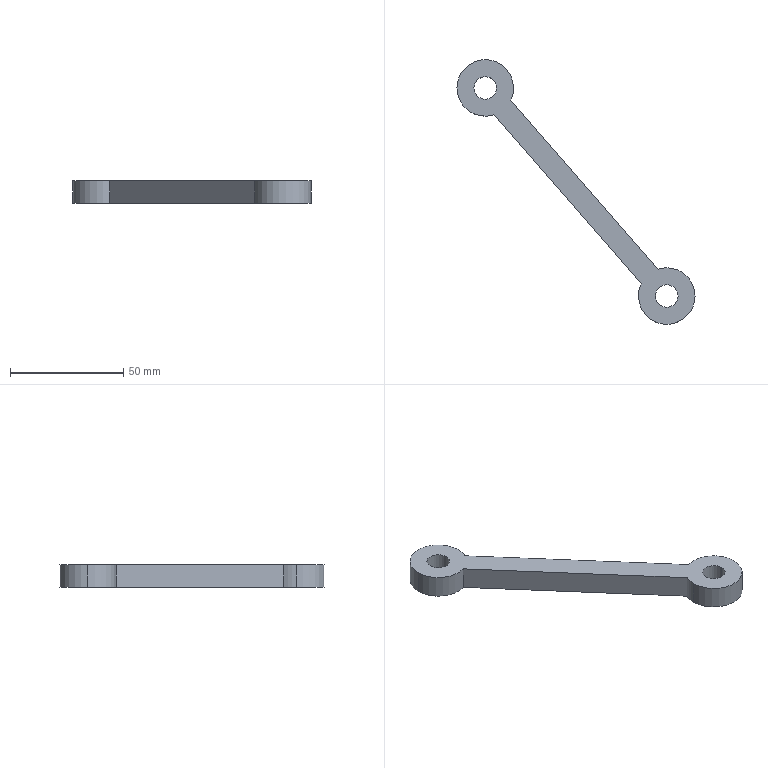Part | SolidWorks | features Extrusion 1 | 1 solid | 14 faces | box 105.181 x 116.951 x 10 mm | volume 18015 mm3 | cylinder 10 | plane 4 | commonest cylinder face diameters 25 x6 10 x4
STEP:
#1=CARTESIAN_POINT('',(762.969,-151.027,-10.));
#2=VERTEX_POINT('',#1);
#3=CARTESIAN_POINT('',(772.969,-151.027,-10.));
#4=VERTEX_POINT('',#3);
#5=CARTESIAN_POINT('',(767.969,-151.027,-10.));
#6=DIRECTION('',(0.,0.,1.));
#7=DIRECTION('',(-1.,0.,0.));
#8=AXIS2_PLACEMENT_3D('',#5,#6,#7);
#9=CIRCLE('',#8,5.);
#10=EDGE_CURVE('',#2,#4,#9,.T.);
#11=ORIENTED_EDGE('',*,*,#10,.F.);
#12=CARTESIAN_POINT('',(762.969,-151.027,0.));
#13=VERTEX_POINT('',#12);
#14=CARTESIAN_POINT('',(762.969,-151.027,-167.291));
#15=DIRECTION('',(0.,0.,1.));
#16=VECTOR('',#15,1000.);
#17=LINE('',#14,#16);
#18=EDGE_CURVE('',#2,#13,#17,.T.);
#19=ORIENTED_EDGE('',*,*,#18,.T.);
#20=CARTESIAN_POINT('',(772.969,-151.027,0.));
#21=VERTEX_POINT('',#20);
#22=CARTESIAN_POINT('',(767.969,-151.027,0.));
#23=DIRECTION('',(0.,0.,1.));
#24=DIRECTION('',(1.,0.,0.));
#25=AXIS2_PLACEMENT_3D('',#22,#23,#24);
#26=CIRCLE('',#25,5.);
#27=EDGE_CURVE('',#13,#21,#26,.T.);
#28=ORIENTED_EDGE('',*,*,#27,.T.);
#29=CARTESIAN_POINT('',(772.969,-151.027,-167.291));
#30=DIRECTION('',(0.,0.,1.));
#31=VECTOR('',#30,1000.);
#32=LINE('',#29,#31);
#33=EDGE_CURVE('',#4,#21,#32,.T.);
#34=ORIENTED_EDGE('',*,*,#33,.F.);
#35=EDGE_LOOP('',(#11,#19,#28,#34));
#36=FACE_OUTER_BOUND('',#35,.T.);
#37=CARTESIAN_POINT('',(767.969,-151.027,-167.291));
#38=DIRECTION('',(0.,0.,1.));
#39=DIRECTION('',(1.,0.,0.));
#40=AXIS2_PLACEMENT_3D('',#37,#38,#39);
#41=CYLINDRICAL_SURFACE('',#40,5.);
#42=ADVANCED_FACE('',(#36),#41,.F.);
#43=CARTESIAN_POINT('',(692.788,-59.076,-10.));
#44=VERTEX_POINT('',#43);
#45=CARTESIAN_POINT('',(682.788,-59.076,-10.));
#46=VERTEX_POINT('',#45);
#47=CARTESIAN_POINT('',(687.788,-59.076,-10.));
#48=DIRECTION('',(0.,0.,-1.));
#49=DIRECTION('',(-1.,0.,0.));
#50=AXIS2_PLACEMENT_3D('',#47,#48,#49);
#51=CIRCLE('',#50,5.);
#52=EDGE_CURVE('',#44,#46,#51,.T.);
#53=ORIENTED_EDGE('',*,*,#52,.T.);
#54=CARTESIAN_POINT('',(682.788,-59.076,0.));
#55=VERTEX_POINT('',#54);
#56=CARTESIAN_POINT('',(682.788,-59.076,-167.291));
#57=DIRECTION('',(0.,0.,1.));
#58=VECTOR('',#57,1000.);
#59=LINE('',#56,#58);
#60=EDGE_CURVE('',#46,#55,#59,.T.);
#61=ORIENTED_EDGE('',*,*,#60,.T.);
#62=CARTESIAN_POINT('',(692.788,-59.076,0.));
#63=VERTEX_POINT('',#62);
#64=CARTESIAN_POINT('',(687.788,-59.076,0.));
#65=DIRECTION('',(0.,0.,-1.));
#66=DIRECTION('',(1.,0.,0.));
#67=AXIS2_PLACEMENT_3D('',#64,#65,#66);
#68=CIRCLE('',#67,5.);
#69=EDGE_CURVE('',#63,#55,#68,.T.);
#70=ORIENTED_EDGE('',*,*,#69,.F.);
#71=CARTESIAN_POINT('',(692.788,-59.076,-167.291));
#72=DIRECTION('',(0.,0.,1.));
#73=VECTOR('',#72,1000.);
#74=LINE('',#71,#73);
#75=EDGE_CURVE('',#44,#63,#74,.T.);
#76=ORIENTED_EDGE('',*,*,#75,.F.);
#77=EDGE_LOOP('',(#53,#61,#70,#76));
#78=FACE_OUTER_BOUND('',#77,.T.);
#79=CARTESIAN_POINT('',(687.788,-59.076,-167.291));
#80=DIRECTION('',(0.,0.,1.));
#81=DIRECTION('',(1.,0.,0.));
#82=AXIS2_PLACEMENT_3D('',#79,#80,#81);
#83=CYLINDRICAL_SURFACE('',#82,5.);
#84=ADVANCED_FACE('',(#78),#83,.F.);
#85=CARTESIAN_POINT('',(756.671,-145.679,-10.));
#86=VERTEX_POINT('',#85);
#87=CARTESIAN_POINT('',(755.469,-151.027,-10.));
#88=VERTEX_POINT('',#87);
#89=CARTESIAN_POINT('',(767.969,-151.027,-10.));
#90=DIRECTION('',(0.,0.,1.));
#91=DIRECTION('',(-1.,0.,0.));
#92=AXIS2_PLACEMENT_3D('',#89,#90,#91);
#93=CIRCLE('',#92,12.5);
#94=EDGE_CURVE('',#86,#88,#93,.T.);
#95=ORIENTED_EDGE('',*,*,#94,.T.);
#96=CARTESIAN_POINT('',(755.469,-151.027,0.));
#97=VERTEX_POINT('',#96);
#98=CARTESIAN_POINT('',(755.469,-151.027,-167.291));
#99=DIRECTION('',(0.,0.,1.));
#100=VECTOR('',#99,1000.);
#101=LINE('',#98,#100);
#102=EDGE_CURVE('',#88,#97,#101,.T.);
#103=ORIENTED_EDGE('',*,*,#102,.T.);
#104=CARTESIAN_POINT('',(756.671,-145.679,0.));
#105=VERTEX_POINT('',#104);
#106=CARTESIAN_POINT('',(767.969,-151.027,0.));
#107=DIRECTION('',(0.,0.,1.));
#108=DIRECTION('',(1.,0.,0.));
#109=AXIS2_PLACEMENT_3D('',#106,#107,#108);
#110=CIRCLE('',#109,12.5);
#111=EDGE_CURVE('',#105,#97,#110,.T.);
#112=ORIENTED_EDGE('',*,*,#111,.F.);
#113=CARTESIAN_POINT('',(756.671,-145.679,-167.291));
#114=DIRECTION('',(0.,0.,1.));
#115=VECTOR('',#114,1000.);
#116=LINE('',#113,#115);
#117=EDGE_CURVE('',#86,#105,#116,.T.);
#118=ORIENTED_EDGE('',*,*,#117,.F.);
#119=EDGE_LOOP('',(#95,#103,#112,#118));
#120=FACE_OUTER_BOUND('',#119,.T.);
#121=CARTESIAN_POINT('',(767.969,-151.027,-167.291));
#122=DIRECTION('',(0.,0.,1.));
#123=DIRECTION('',(1.,0.,0.));
#124=AXIS2_PLACEMENT_3D('',#121,#122,#123);
#125=CYLINDRICAL_SURFACE('',#124,12.5);
#126=ADVANCED_FACE('',(#120),#125,.T.);
#127=ORIENTED_EDGE('',*,*,#102,.F.);
#128=CARTESIAN_POINT('',(780.469,-151.027,-10.));
#129=VERTEX_POINT('',#128);
#130=CARTESIAN_POINT('',(767.969,-151.027,-10.));
#131=DIRECTION('',(0.,0.,1.));
#132=DIRECTION('',(-1.,0.,0.));
#133=AXIS2_PLACEMENT_3D('',#130,#131,#132);
#134=CIRCLE('',#133,12.5);
#135=EDGE_CURVE('',#88,#129,#134,.T.);
#136=ORIENTED_EDGE('',*,*,#135,.T.);
#137=CARTESIAN_POINT('',(780.469,-151.027,0.));
#138=VERTEX_POINT('',#137);
#139=CARTESIAN_POINT('',(780.469,-151.027,-167.291));
#140=DIRECTION('',(0.,0.,1.));
#141=VECTOR('',#140,1000.);
#142=LINE('',#139,#141);
#143=EDGE_CURVE('',#129,#138,#142,.T.);
#144=ORIENTED_EDGE('',*,*,#143,.T.);
#145=CARTESIAN_POINT('',(767.969,-151.027,0.));
#146=DIRECTION('',(0.,0.,1.));
#147=DIRECTION('',(1.,0.,0.));
#148=AXIS2_PLACEMENT_3D('',#145,#146,#147);
#149=CIRCLE('',#148,12.5);
#150=EDGE_CURVE('',#97,#138,#149,.T.);
#151=ORIENTED_EDGE('',*,*,#150,.F.);
#152=EDGE_LOOP('',(#127,#136,#144,#151));
#153=FACE_OUTER_BOUND('',#152,.T.);
#154=CARTESIAN_POINT('',(767.969,-151.027,-167.291));
#155=DIRECTION('',(0.,0.,1.));
#156=DIRECTION('',(1.,0.,0.));
#157=AXIS2_PLACEMENT_3D('',#154,#155,#156);
#158=CYLINDRICAL_SURFACE('',#157,12.5);
#159=ADVANCED_FACE('',(#153),#158,.T.);
#160=CARTESIAN_POINT('',(700.288,-59.076,-10.));
#161=VERTEX_POINT('',#160);
#162=CARTESIAN_POINT('',(675.288,-59.076,-10.));
#163=VERTEX_POINT('',#162);
#164=CARTESIAN_POINT('',(687.788,-59.076,-10.));
#165=DIRECTION('',(0.,0.,1.));
#166=DIRECTION('',(-1.,0.,0.));
#167=AXIS2_PLACEMENT_3D('',#164,#165,#166);
#168=CIRCLE('',#167,12.5);
#169=EDGE_CURVE('',#161,#163,#168,.T.);
#170=ORIENTED_EDGE('',*,*,#169,.T.);
#171=CARTESIAN_POINT('',(675.288,-59.076,0.));
#172=VERTEX_POINT('',#171);
#173=CARTESIAN_POINT('',(675.288,-59.076,-167.291));
#174=DIRECTION('',(0.,0.,1.));
#175=VECTOR('',#174,1000.);
#176=LINE('',#173,#175);
#177=EDGE_CURVE('',#163,#172,#176,.T.);
#178=ORIENTED_EDGE('',*,*,#177,.T.);
#179=CARTESIAN_POINT('',(700.288,-59.076,0.));
#180=VERTEX_POINT('',#179);
#181=CARTESIAN_POINT('',(687.788,-59.076,0.));
#182=DIRECTION('',(0.,0.,1.));
#183=DIRECTION('',(1.,0.,0.));
#184=AXIS2_PLACEMENT_3D('',#181,#182,#183);
#185=CIRCLE('',#184,12.5);
#186=EDGE_CURVE('',#180,#172,#185,.T.);
#187=ORIENTED_EDGE('',*,*,#186,.F.);
#188=CARTESIAN_POINT('',(700.288,-59.076,-167.291));
#189=DIRECTION('',(0.,0.,1.));
#190=VECTOR('',#189,1000.);
#191=LINE('',#188,#190);
#192=EDGE_CURVE('',#161,#180,#191,.T.);
#193=ORIENTED_EDGE('',*,*,#192,.F.);
#194=EDGE_LOOP('',(#170,#178,#187,#193));
#195=FACE_OUTER_BOUND('',#194,.T.);
#196=CARTESIAN_POINT('',(687.788,-59.076,-167.291));
#197=DIRECTION('',(0.,0.,1.));
#198=DIRECTION('',(1.,0.,0.));
#199=AXIS2_PLACEMENT_3D('',#196,#197,#198);
#200=CYLINDRICAL_SURFACE('',#199,12.5);
#201=ADVANCED_FACE('',(#195),#200,.T.);
#202=CARTESIAN_POINT('',(699.086,-64.425,-10.));
#203=VERTEX_POINT('',#202);
#204=CARTESIAN_POINT('',(687.788,-59.076,-10.));
#205=DIRECTION('',(0.,0.,1.));
#206=DIRECTION('',(-1.,0.,0.));
#207=AXIS2_PLACEMENT_3D('',#204,#205,#206);
#208=CIRCLE('',#207,12.5);
#209=EDGE_CURVE('',#203,#161,#208,.T.);
#210=ORIENTED_EDGE('',*,*,#209,.T.);
#211=ORIENTED_EDGE('',*,*,#192,.T.);
#212=CARTESIAN_POINT('',(699.086,-64.425,0.));
#213=VERTEX_POINT('',#212);
#214=CARTESIAN_POINT('',(687.788,-59.076,0.));
#215=DIRECTION('',(0.,0.,1.));
#216=DIRECTION('',(1.,0.,0.));
#217=AXIS2_PLACEMENT_3D('',#214,#215,#216);
#218=CIRCLE('',#217,12.5);
#219=EDGE_CURVE('',#213,#180,#218,.T.);
#220=ORIENTED_EDGE('',*,*,#219,.F.);
#221=CARTESIAN_POINT('',(699.086,-64.425,-167.291));
#222=DIRECTION('',(0.,0.,1.));
#223=VECTOR('',#222,1000.);
#224=LINE('',#221,#223);
#225=EDGE_CURVE('',#203,#213,#224,.T.);
#226=ORIENTED_EDGE('',*,*,#225,.F.);
#227=EDGE_LOOP('',(#210,#211,#220,#226));
#228=FACE_OUTER_BOUND('',#227,.T.);
#229=CARTESIAN_POINT('',(687.788,-59.076,-167.291));
#230=DIRECTION('',(0.,0.,1.));
#231=DIRECTION('',(1.,0.,0.));
#232=AXIS2_PLACEMENT_3D('',#229,#230,#231);
#233=CYLINDRICAL_SURFACE('',#232,12.5);
#234=ADVANCED_FACE('',(#228),#233,.T.);
#235=ORIENTED_EDGE('',*,*,#177,.F.);
#236=CARTESIAN_POINT('',(691.549,-70.997,-10.));
#237=VERTEX_POINT('',#236);
#238=CARTESIAN_POINT('',(687.788,-59.076,-10.));
#239=DIRECTION('',(0.,0.,1.));
#240=DIRECTION('',(-1.,0.,0.));
#241=AXIS2_PLACEMENT_3D('',#238,#239,#240);
#242=CIRCLE('',#241,12.5);
#243=EDGE_CURVE('',#163,#237,#242,.T.);
#244=ORIENTED_EDGE('',*,*,#243,.T.);
#245=CARTESIAN_POINT('',(691.549,-70.997,0.));
#246=VERTEX_POINT('',#245);
#247=CARTESIAN_POINT('',(691.549,-70.997,-167.291));
#248=DIRECTION('',(0.,0.,1.));
#249=VECTOR('',#248,1000.);
#250=LINE('',#247,#249);
#251=EDGE_CURVE('',#237,#246,#250,.T.);
#252=ORIENTED_EDGE('',*,*,#251,.T.);
#253=CARTESIAN_POINT('',(687.788,-59.076,0.));
#254=DIRECTION('',(0.,0.,1.));
#255=DIRECTION('',(1.,0.,0.));
#256=AXIS2_PLACEMENT_3D('',#253,#254,#255);
#257=CIRCLE('',#256,12.5);
#258=EDGE_CURVE('',#172,#246,#257,.T.);
#259=ORIENTED_EDGE('',*,*,#258,.F.);
#260=EDGE_LOOP('',(#235,#244,#252,#259));
#261=FACE_OUTER_BOUND('',#260,.T.);
#262=CARTESIAN_POINT('',(687.788,-59.076,-167.291));
#263=DIRECTION('',(0.,0.,1.));
#264=DIRECTION('',(1.,0.,0.));
#265=AXIS2_PLACEMENT_3D('',#262,#263,#264);
#266=CYLINDRICAL_SURFACE('',#265,12.5);
#267=ADVANCED_FACE('',(#261),#266,.T.);
#268=CARTESIAN_POINT('',(764.208,-139.107,-10.));
#269=VERTEX_POINT('',#268);
#270=CARTESIAN_POINT('',(764.208,-139.107,0.));
#271=VERTEX_POINT('',#270);
#272=CARTESIAN_POINT('',(764.208,-139.107,-167.291));
#273=DIRECTION('',(0.,0.,1.));
#274=VECTOR('',#273,1000.);
#275=LINE('',#272,#274);
#276=EDGE_CURVE('',#269,#271,#275,.T.);
#277=ORIENTED_EDGE('',*,*,#276,.F.);
#278=CARTESIAN_POINT('',(365.211,318.462,-10.));
#279=DIRECTION('',(-0.6572,0.7537,0.));
#280=VECTOR('',#279,1000.);
#281=LINE('',#278,#280);
#282=EDGE_CURVE('',#269,#203,#281,.T.);
#283=ORIENTED_EDGE('',*,*,#282,.T.);
#284=ORIENTED_EDGE('',*,*,#225,.T.);
#285=CARTESIAN_POINT('',(365.211,318.462,0.));
#286=DIRECTION('',(-0.6572,0.7537,0.));
#287=VECTOR('',#286,1000.);
#288=LINE('',#285,#287);
#289=EDGE_CURVE('',#271,#213,#288,.T.);
#290=ORIENTED_EDGE('',*,*,#289,.F.);
#291=EDGE_LOOP('',(#277,#283,#284,#290));
#292=FACE_OUTER_BOUND('',#291,.T.);
#293=CARTESIAN_POINT('',(365.211,318.462,-167.291));
#294=DIRECTION('',(0.7537,0.6572,0.));
#295=DIRECTION('',(-0.6572,0.7537,0.));
#296=AXIS2_PLACEMENT_3D('',#293,#294,#295);
#297=PLANE('',#296);
#298=ADVANCED_FACE('',(#292),#297,.T.);
#299=ORIENTED_EDGE('',*,*,#143,.F.);
#300=CARTESIAN_POINT('',(767.969,-151.027,-10.));
#301=DIRECTION('',(0.,0.,1.));
#302=DIRECTION('',(-1.,0.,0.));
#303=AXIS2_PLACEMENT_3D('',#300,#301,#302);
#304=CIRCLE('',#303,12.5);
#305=EDGE_CURVE('',#129,#269,#304,.T.);
#306=ORIENTED_EDGE('',*,*,#305,.T.);
#307=ORIENTED_EDGE('',*,*,#276,.T.);
#308=CARTESIAN_POINT('',(767.969,-151.027,0.));
#309=DIRECTION('',(0.,0.,1.));
#310=DIRECTION('',(1.,0.,0.));
#311=AXIS2_PLACEMENT_3D('',#308,#309,#310);
#312=CIRCLE('',#311,12.5);
#313=EDGE_CURVE('',#138,#271,#312,.T.);
#314=ORIENTED_EDGE('',*,*,#313,.F.);
#315=EDGE_LOOP('',(#299,#306,#307,#314));
#316=FACE_OUTER_BOUND('',#315,.T.);
#317=CARTESIAN_POINT('',(767.969,-151.027,-167.291));
#318=DIRECTION('',(0.,0.,1.));
#319=DIRECTION('',(1.,0.,0.));
#320=AXIS2_PLACEMENT_3D('',#317,#318,#319);
#321=CYLINDRICAL_SURFACE('',#320,12.5);
#322=ADVANCED_FACE('',(#316),#321,.T.);
#323=ORIENTED_EDGE('',*,*,#60,.F.);
#324=CARTESIAN_POINT('',(687.788,-59.076,-10.));
#325=DIRECTION('',(0.,0.,-1.));
#326=DIRECTION('',(-1.,0.,0.));
#327=AXIS2_PLACEMENT_3D('',#324,#325,#326);
#328=CIRCLE('',#327,5.);
#329=EDGE_CURVE('',#46,#44,#328,.T.);
#330=ORIENTED_EDGE('',*,*,#329,.T.);
#331=ORIENTED_EDGE('',*,*,#75,.T.);
#332=CARTESIAN_POINT('',(687.788,-59.076,0.));
#333=DIRECTION('',(0.,0.,-1.));
#334=DIRECTION('',(1.,0.,0.));
#335=AXIS2_PLACEMENT_3D('',#332,#333,#334);
#336=CIRCLE('',#335,5.);
#337=EDGE_CURVE('',#55,#63,#336,.T.);
#338=ORIENTED_EDGE('',*,*,#337,.F.);
#339=EDGE_LOOP('',(#323,#330,#331,#338));
#340=FACE_OUTER_BOUND('',#339,.T.);
#341=CARTESIAN_POINT('',(687.788,-59.076,-167.291));
#342=DIRECTION('',(0.,0.,1.));
#343=DIRECTION('',(1.,0.,0.));
#344=AXIS2_PLACEMENT_3D('',#341,#342,#343);
#345=CYLINDRICAL_SURFACE('',#344,5.);
#346=ADVANCED_FACE('',(#340),#345,.F.);
#347=ORIENTED_EDGE('',*,*,#251,.F.);
#348=CARTESIAN_POINT('',(357.674,311.89,-10.));
#349=DIRECTION('',(0.6572,-0.7537,0.));
#350=VECTOR('',#349,1000.);
#351=LINE('',#348,#350);
#352=EDGE_CURVE('',#237,#86,#351,.T.);
#353=ORIENTED_EDGE('',*,*,#352,.T.);
#354=ORIENTED_EDGE('',*,*,#117,.T.);
#355=CARTESIAN_POINT('',(357.674,311.89,0.));
#356=DIRECTION('',(0.6572,-0.7537,0.));
#357=VECTOR('',#356,1000.);
#358=LINE('',#355,#357);
#359=EDGE_CURVE('',#246,#105,#358,.T.);
#360=ORIENTED_EDGE('',*,*,#359,.F.);
#361=EDGE_LOOP('',(#347,#353,#354,#360));
#362=FACE_OUTER_BOUND('',#361,.T.);
#363=CARTESIAN_POINT('',(357.674,311.89,-167.291));
#364=DIRECTION('',(-0.7537,-0.6572,0.));
#365=DIRECTION('',(0.6572,-0.7537,0.));
#366=AXIS2_PLACEMENT_3D('',#363,#364,#365);
#367=PLANE('',#366);
#368=ADVANCED_FACE('',(#362),#367,.T.);
#369=ORIENTED_EDGE('',*,*,#18,.F.);
#370=CARTESIAN_POINT('',(767.969,-151.027,-10.));
#371=DIRECTION('',(0.,0.,1.));
#372=DIRECTION('',(-1.,0.,0.));
#373=AXIS2_PLACEMENT_3D('',#370,#371,#372);
#374=CIRCLE('',#373,5.);
#375=EDGE_CURVE('',#4,#2,#374,.T.);
#376=ORIENTED_EDGE('',*,*,#375,.F.);
#377=ORIENTED_EDGE('',*,*,#33,.T.);
#378=CARTESIAN_POINT('',(767.969,-151.027,0.));
#379=DIRECTION('',(0.,0.,1.));
#380=DIRECTION('',(1.,0.,0.));
#381=AXIS2_PLACEMENT_3D('',#378,#379,#380);
#382=CIRCLE('',#381,5.);
#383=EDGE_CURVE('',#21,#13,#382,.T.);
#384=ORIENTED_EDGE('',*,*,#383,.T.);
#385=EDGE_LOOP('',(#369,#376,#377,#384));
#386=FACE_OUTER_BOUND('',#385,.T.);
#387=CARTESIAN_POINT('',(767.969,-151.027,-167.291));
#388=DIRECTION('',(0.,0.,1.));
#389=DIRECTION('',(1.,0.,0.));
#390=AXIS2_PLACEMENT_3D('',#387,#388,#389);
#391=CYLINDRICAL_SURFACE('',#390,5.);
#392=ADVANCED_FACE('',(#386),#391,.F.);
#393=ORIENTED_EDGE('',*,*,#219,.T.);
#394=ORIENTED_EDGE('',*,*,#186,.T.);
#395=ORIENTED_EDGE('',*,*,#258,.T.);
#396=ORIENTED_EDGE('',*,*,#359,.T.);
#397=ORIENTED_EDGE('',*,*,#111,.T.);
#398=ORIENTED_EDGE('',*,*,#150,.T.);
#399=ORIENTED_EDGE('',*,*,#313,.T.);
#400=ORIENTED_EDGE('',*,*,#289,.T.);
#401=EDGE_LOOP('',(#393,#394,#395,#396,#397,#398,#399,#400));
#402=FACE_OUTER_BOUND('',#401,.T.);
#403=ORIENTED_EDGE('',*,*,#69,.T.);
#404=ORIENTED_EDGE('',*,*,#337,.T.);
#405=EDGE_LOOP('',(#403,#404));
#406=FACE_BOUND('',#405,.T.);
#407=ORIENTED_EDGE('',*,*,#383,.F.);
#408=ORIENTED_EDGE('',*,*,#27,.F.);
#409=EDGE_LOOP('',(#407,#408));
#410=FACE_BOUND('',#409,.T.);
#411=CARTESIAN_POINT('',(0.,0.,0.));
#412=DIRECTION('',(0.,0.,1.));
#413=DIRECTION('',(1.,0.,0.));
#414=AXIS2_PLACEMENT_3D('',#411,#412,#413);
#415=PLANE('',#414);
#416=ADVANCED_FACE('',(#402,#406,#410),#415,.T.);
#417=ORIENTED_EDGE('',*,*,#52,.F.);
#418=ORIENTED_EDGE('',*,*,#329,.F.);
#419=EDGE_LOOP('',(#417,#418));
#420=FACE_BOUND('',#419,.T.);
#421=ORIENTED_EDGE('',*,*,#209,.F.);
#422=ORIENTED_EDGE('',*,*,#282,.F.);
#423=ORIENTED_EDGE('',*,*,#305,.F.);
#424=ORIENTED_EDGE('',*,*,#135,.F.);
#425=ORIENTED_EDGE('',*,*,#94,.F.);
#426=ORIENTED_EDGE('',*,*,#352,.F.);
#427=ORIENTED_EDGE('',*,*,#243,.F.);
#428=ORIENTED_EDGE('',*,*,#169,.F.);
#429=EDGE_LOOP('',(#421,#422,#423,#424,#425,#426,#427,#428));
#430=FACE_OUTER_BOUND('',#429,.T.);
#431=ORIENTED_EDGE('',*,*,#375,.T.);
#432=ORIENTED_EDGE('',*,*,#10,.T.);
#433=EDGE_LOOP('',(#431,#432));
#434=FACE_BOUND('',#433,.T.);
#435=CARTESIAN_POINT('',(760.739,-142.737,-10.));
#436=DIRECTION('',(0.,0.,-1.));
#437=DIRECTION('',(-0.7537,-0.6572,0.));
#438=AXIS2_PLACEMENT_3D('',#435,#436,#437);
#439=PLANE('',#438);
#440=ADVANCED_FACE('',(#420,#430,#434),#439,.T.);
#441=CLOSED_SHELL('',(#42,#84,#126,#159,#201,#234,#267,#298,#322,#346,#368,#392,#416,#440));
#442=MANIFOLD_SOLID_BREP('',#441);
#443=CARTESIAN_POINT('',(0.,0.,0.));
#444=DIRECTION('',(0.,0.,1.));
#445=DIRECTION('',(1.,0.,0.));
#446=AXIS2_PLACEMENT_3D('',#443,#444,#445);
#447=(LENGTH_UNIT()NAMED_UNIT(*)SI_UNIT(.MILLI.,.METRE.));
#448=UNCERTAINTY_MEASURE_WITH_UNIT(LENGTH_MEASURE(0.00001),#447,'','');
#449=(NAMED_UNIT(*)PLANE_ANGLE_UNIT()SI_UNIT($,.RADIAN.));
#450=(NAMED_UNIT(*)SI_UNIT($,.STERADIAN.)SOLID_ANGLE_UNIT());
#451=(GEOMETRIC_REPRESENTATION_CONTEXT(3)GLOBAL_UNCERTAINTY_ASSIGNED_CONTEXT((#448))GLOBAL_UNIT_ASSIGNED_CONTEXT((#447,#449,#450))REPRESENTATION_CONTEXT('',''));
#452=ADVANCED_BREP_SHAPE_REPRESENTATION('',(#442,#446),#451);